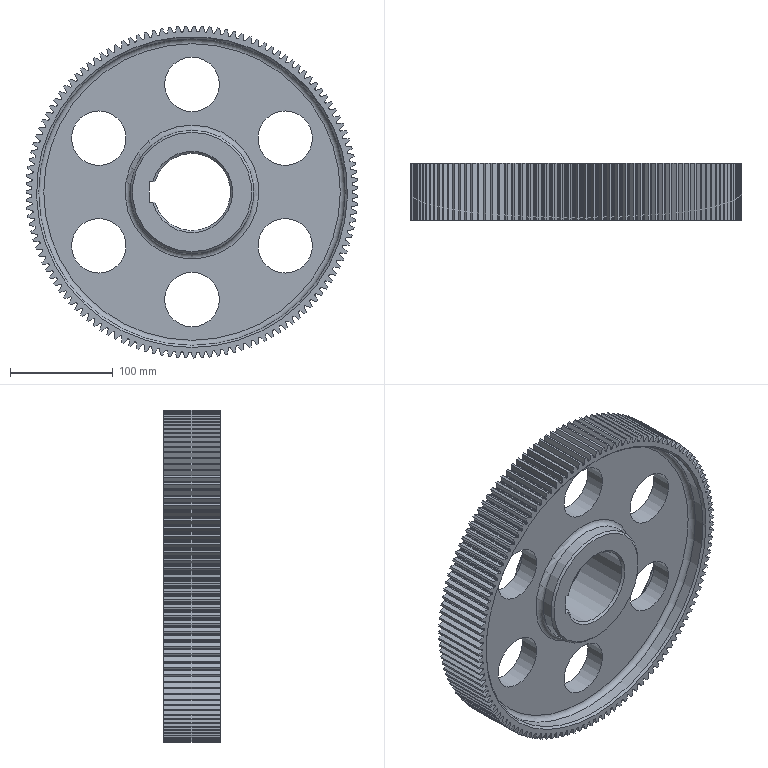Part | NX | features BREP 127, META 127, DATUM_CSYS 10, SKETCH 9, EXTRACT_DATUM_AXIS 8, HOLE PACKAGE 7, SIMPLE HOLE 7, EXTRACT_FACE 6, Instance Feature 6, EXTRUDE 3, EXTRACT_DATUM_PLANE 2, BLEND 1, CHAMFER 1, CYLINDER 1, FSET 1, Mirror Feature 1, Pattern Feature 1 | 1 solid | 792 faces | box 322.473 x 55 x 322.494 mm | volume 1796167 mm3 | spline 635 | cylinder 138 | plane 9 | cone 6 | torus 4 | commonest cylinder face diameters 311.25 x127 53 x6 120 x2 298 x2 75 x1